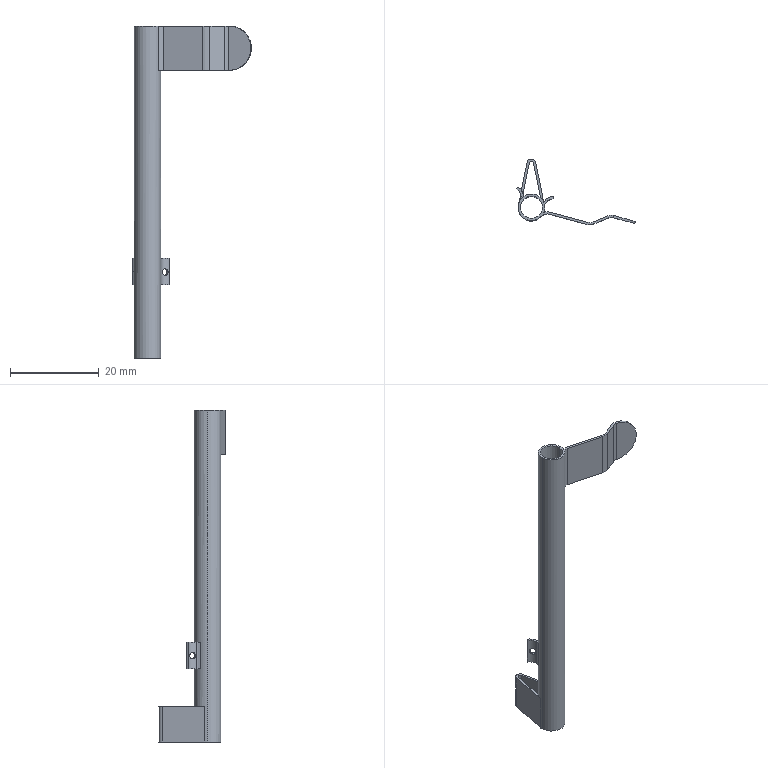Part | SolidWorks | features BossThin 3, 3DProfileFeature 1, Extrusion 1, Fillet 1, HoleWzd 1, ICE 1 | 1 solid | 43 faces | box 26.854 x 14.962 x 75 mm | volume 843.538 mm3 | plane 22 | cylinder 21 | commonest cylinder face diameters 5 x6 4 x5 1.5 x4 6 x2 1 x1 2 x1